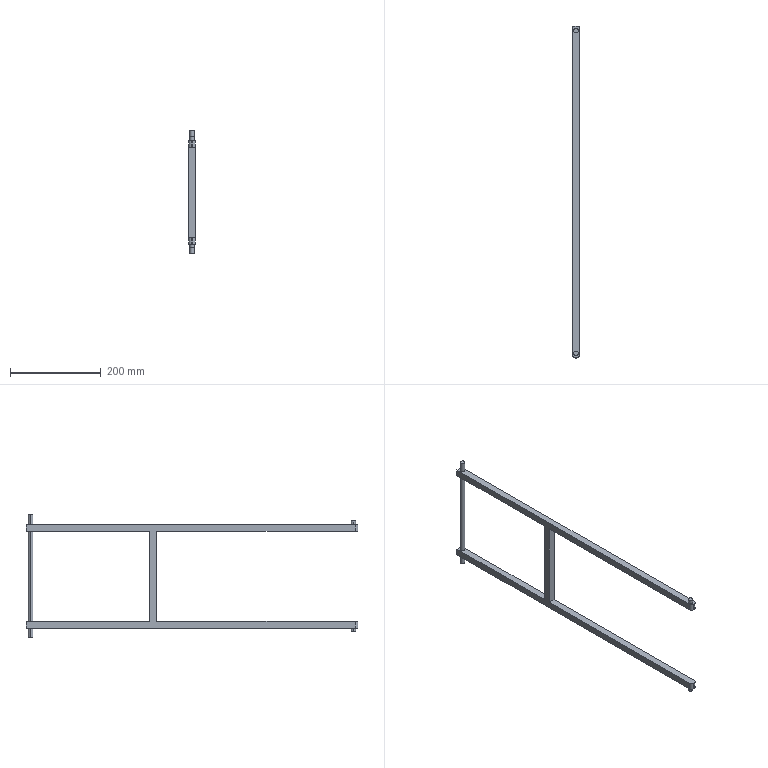Part | SolidWorks | features ICE 5, Extrusion 1, Fillet 1 | 1 solid | 32 faces | box 15 x 730 x 270 mm | volume 392693 mm3 | plane 18 | cylinder 14 | commonest cylinder face diameters 10 x10 12 x4
STEP:
#1=CARTESIAN_POINT('',(-5.,720.,-27.5));
#2=VERTEX_POINT('',#1);
#3=CARTESIAN_POINT('',(5.,720.,-27.5));
#4=VERTEX_POINT('',#3);
#5=CARTESIAN_POINT('',(0.,720.,-27.5));
#6=DIRECTION('',(0.,0.,-1.));
#7=DIRECTION('',(-1.,0.,0.));
#8=AXIS2_PLACEMENT_3D('',#5,#6,#7);
#9=CIRCLE('',#8,5.);
#10=EDGE_CURVE('',#2,#4,#9,.T.);
#11=ORIENTED_EDGE('',*,*,#10,.F.);
#12=CARTESIAN_POINT('',(-5.,720.,-7.5));
#13=VERTEX_POINT('',#12);
#14=CARTESIAN_POINT('',(-5.,720.,-27.5));
#15=DIRECTION('',(0.,0.,1.));
#16=VECTOR('',#15,1000.);
#17=LINE('',#14,#16);
#18=EDGE_CURVE('',#2,#13,#17,.T.);
#19=ORIENTED_EDGE('',*,*,#18,.T.);
#20=CARTESIAN_POINT('',(5.,720.,-7.5));
#21=VERTEX_POINT('',#20);
#22=CARTESIAN_POINT('',(0.,720.,-7.5));
#23=DIRECTION('',(0.,0.,-1.));
#24=DIRECTION('',(1.,0.,0.));
#25=AXIS2_PLACEMENT_3D('',#22,#23,#24);
#26=CIRCLE('',#25,5.);
#27=EDGE_CURVE('',#13,#21,#26,.T.);
#28=ORIENTED_EDGE('',*,*,#27,.T.);
#29=CARTESIAN_POINT('',(5.,720.,-27.5));
#30=DIRECTION('',(0.,0.,1.));
#31=VECTOR('',#30,1000.);
#32=LINE('',#29,#31);
#33=EDGE_CURVE('',#4,#21,#32,.T.);
#34=ORIENTED_EDGE('',*,*,#33,.F.);
#35=EDGE_LOOP('',(#11,#19,#28,#34));
#36=FACE_OUTER_BOUND('',#35,.T.);
#37=CARTESIAN_POINT('',(0.,720.,-27.5));
#38=DIRECTION('',(0.,0.,1.));
#39=DIRECTION('',(1.,0.,0.));
#40=AXIS2_PLACEMENT_3D('',#37,#38,#39);
#41=CYLINDRICAL_SURFACE('',#40,5.);
#42=ADVANCED_FACE('',(#36),#41,.T.);
#43=CARTESIAN_POINT('',(5.,720.,7.5));
#44=VERTEX_POINT('',#43);
#45=CARTESIAN_POINT('',(-5.,720.,7.5));
#46=VERTEX_POINT('',#45);
#47=CARTESIAN_POINT('',(0.,720.,7.5));
#48=DIRECTION('',(0.,0.,1.));
#49=DIRECTION('',(-1.,0.,0.));
#50=AXIS2_PLACEMENT_3D('',#47,#48,#49);
#51=CIRCLE('',#50,5.);
#52=EDGE_CURVE('',#44,#46,#51,.T.);
#53=ORIENTED_EDGE('',*,*,#52,.T.);
#54=CARTESIAN_POINT('',(-5.,720.,205.5));
#55=VERTEX_POINT('',#54);
#56=CARTESIAN_POINT('',(-5.,720.,-27.5));
#57=DIRECTION('',(0.,0.,1.));
#58=VECTOR('',#57,1000.);
#59=LINE('',#56,#58);
#60=EDGE_CURVE('',#46,#55,#59,.T.);
#61=ORIENTED_EDGE('',*,*,#60,.T.);
#62=CARTESIAN_POINT('',(5.,720.,205.5));
#63=VERTEX_POINT('',#62);
#64=CARTESIAN_POINT('',(0.,720.,205.5));
#65=DIRECTION('',(0.,0.,-1.));
#66=DIRECTION('',(1.,0.,0.));
#67=AXIS2_PLACEMENT_3D('',#64,#65,#66);
#68=CIRCLE('',#67,5.);
#69=EDGE_CURVE('',#55,#63,#68,.T.);
#70=ORIENTED_EDGE('',*,*,#69,.T.);
#71=CARTESIAN_POINT('',(5.,720.,-27.5));
#72=DIRECTION('',(0.,0.,1.));
#73=VECTOR('',#72,1000.);
#74=LINE('',#71,#73);
#75=EDGE_CURVE('',#44,#63,#74,.T.);
#76=ORIENTED_EDGE('',*,*,#75,.F.);
#77=EDGE_LOOP('',(#53,#61,#70,#76));
#78=FACE_OUTER_BOUND('',#77,.T.);
#79=CARTESIAN_POINT('',(0.,720.,-27.5));
#80=DIRECTION('',(0.,0.,1.));
#81=DIRECTION('',(1.,0.,0.));
#82=AXIS2_PLACEMENT_3D('',#79,#80,#81);
#83=CYLINDRICAL_SURFACE('',#82,5.);
#84=ADVANCED_FACE('',(#78),#83,.T.);
#85=CARTESIAN_POINT('',(-5.,720.,220.5));
#86=VERTEX_POINT('',#85);
#87=CARTESIAN_POINT('',(5.,720.,220.5));
#88=VERTEX_POINT('',#87);
#89=CARTESIAN_POINT('',(0.,720.,220.5));
#90=DIRECTION('',(0.,0.,-1.));
#91=DIRECTION('',(1.,0.,0.));
#92=AXIS2_PLACEMENT_3D('',#89,#90,#91);
#93=CIRCLE('',#92,5.);
#94=EDGE_CURVE('',#86,#88,#93,.T.);
#95=ORIENTED_EDGE('',*,*,#94,.F.);
#96=CARTESIAN_POINT('',(-5.,720.,242.5));
#97=VERTEX_POINT('',#96);
#98=CARTESIAN_POINT('',(-5.,720.,-27.5));
#99=DIRECTION('',(0.,0.,1.));
#100=VECTOR('',#99,1000.);
#101=LINE('',#98,#100);
#102=EDGE_CURVE('',#86,#97,#101,.T.);
#103=ORIENTED_EDGE('',*,*,#102,.T.);
#104=CARTESIAN_POINT('',(5.,720.,242.5));
#105=VERTEX_POINT('',#104);
#106=CARTESIAN_POINT('',(0.,720.,242.5));
#107=DIRECTION('',(0.,0.,-1.));
#108=DIRECTION('',(-1.,0.,0.));
#109=AXIS2_PLACEMENT_3D('',#106,#107,#108);
#110=CIRCLE('',#109,5.);
#111=EDGE_CURVE('',#97,#105,#110,.T.);
#112=ORIENTED_EDGE('',*,*,#111,.T.);
#113=CARTESIAN_POINT('',(5.,720.,-27.5));
#114=DIRECTION('',(0.,0.,1.));
#115=VECTOR('',#114,1000.);
#116=LINE('',#113,#115);
#117=EDGE_CURVE('',#88,#105,#116,.T.);
#118=ORIENTED_EDGE('',*,*,#117,.F.);
#119=EDGE_LOOP('',(#95,#103,#112,#118));
#120=FACE_OUTER_BOUND('',#119,.T.);
#121=CARTESIAN_POINT('',(0.,720.,-27.5));
#122=DIRECTION('',(0.,0.,1.));
#123=DIRECTION('',(1.,0.,0.));
#124=AXIS2_PLACEMENT_3D('',#121,#122,#123);
#125=CYLINDRICAL_SURFACE('',#124,5.);
#126=ADVANCED_FACE('',(#120),#125,.T.);
#127=CARTESIAN_POINT('',(5.,10.,228.5));
#128=VERTEX_POINT('',#127);
#129=CARTESIAN_POINT('',(-5.,10.,228.5));
#130=VERTEX_POINT('',#129);
#131=CARTESIAN_POINT('',(0.,10.,228.5));
#132=DIRECTION('',(0.,0.,1.));
#133=DIRECTION('',(1.,0.,0.));
#134=AXIS2_PLACEMENT_3D('',#131,#132,#133);
#135=CIRCLE('',#134,5.);
#136=EDGE_CURVE('',#128,#130,#135,.T.);
#137=ORIENTED_EDGE('',*,*,#136,.F.);
#138=CARTESIAN_POINT('',(5.,10.,220.5));
#139=VERTEX_POINT('',#138);
#140=CARTESIAN_POINT('',(5.,10.,228.5));
#141=DIRECTION('',(0.,0.,-1.));
#142=VECTOR('',#141,1000.);
#143=LINE('',#140,#142);
#144=EDGE_CURVE('',#128,#139,#143,.T.);
#145=ORIENTED_EDGE('',*,*,#144,.T.);
#146=CARTESIAN_POINT('',(-5.,10.,220.5));
#147=VERTEX_POINT('',#146);
#148=CARTESIAN_POINT('',(0.,10.,220.5));
#149=DIRECTION('',(0.,0.,1.));
#150=DIRECTION('',(1.,0.,0.));
#151=AXIS2_PLACEMENT_3D('',#148,#149,#150);
#152=CIRCLE('',#151,5.);
#153=EDGE_CURVE('',#139,#147,#152,.T.);
#154=ORIENTED_EDGE('',*,*,#153,.T.);
#155=CARTESIAN_POINT('',(-5.,10.,228.5));
#156=DIRECTION('',(0.,0.,-1.));
#157=VECTOR('',#156,1000.);
#158=LINE('',#155,#157);
#159=EDGE_CURVE('',#130,#147,#158,.T.);
#160=ORIENTED_EDGE('',*,*,#159,.F.);
#161=EDGE_LOOP('',(#137,#145,#154,#160));
#162=FACE_OUTER_BOUND('',#161,.T.);
#163=CARTESIAN_POINT('',(0.,10.,228.5));
#164=DIRECTION('',(0.,0.,-1.));
#165=DIRECTION('',(-1.,0.,0.));
#166=AXIS2_PLACEMENT_3D('',#163,#164,#165);
#167=CYLINDRICAL_SURFACE('',#166,5.);
#168=ADVANCED_FACE('',(#162),#167,.T.);
#169=CARTESIAN_POINT('',(-5.,10.,-15.5));
#170=VERTEX_POINT('',#169);
#171=CARTESIAN_POINT('',(5.,10.,-15.5));
#172=VERTEX_POINT('',#171);
#173=CARTESIAN_POINT('',(0.,10.,-15.5));
#174=DIRECTION('',(0.,0.,-1.));
#175=DIRECTION('',(-1.,0.,0.));
#176=AXIS2_PLACEMENT_3D('',#173,#174,#175);
#177=CIRCLE('',#176,5.);
#178=EDGE_CURVE('',#170,#172,#177,.T.);
#179=ORIENTED_EDGE('',*,*,#178,.F.);
#180=CARTESIAN_POINT('',(-5.,10.,-7.5));
#181=VERTEX_POINT('',#180);
#182=CARTESIAN_POINT('',(-5.,10.,-15.5));
#183=DIRECTION('',(0.,0.,1.));
#184=VECTOR('',#183,1000.);
#185=LINE('',#182,#184);
#186=EDGE_CURVE('',#170,#181,#185,.T.);
#187=ORIENTED_EDGE('',*,*,#186,.T.);
#188=CARTESIAN_POINT('',(5.,10.,-7.5));
#189=VERTEX_POINT('',#188);
#190=CARTESIAN_POINT('',(0.,10.,-7.5));
#191=DIRECTION('',(0.,0.,-1.));
#192=DIRECTION('',(1.,0.,0.));
#193=AXIS2_PLACEMENT_3D('',#190,#191,#192);
#194=CIRCLE('',#193,5.);
#195=EDGE_CURVE('',#181,#189,#194,.T.);
#196=ORIENTED_EDGE('',*,*,#195,.T.);
#197=CARTESIAN_POINT('',(5.,10.,-15.5));
#198=DIRECTION('',(0.,0.,1.));
#199=VECTOR('',#198,1000.);
#200=LINE('',#197,#199);
#201=EDGE_CURVE('',#172,#189,#200,.T.);
#202=ORIENTED_EDGE('',*,*,#201,.F.);
#203=EDGE_LOOP('',(#179,#187,#196,#202));
#204=FACE_OUTER_BOUND('',#203,.T.);
#205=CARTESIAN_POINT('',(0.,10.,-15.5));
#206=DIRECTION('',(0.,0.,1.));
#207=DIRECTION('',(1.,0.,0.));
#208=AXIS2_PLACEMENT_3D('',#205,#206,#207);
#209=CYLINDRICAL_SURFACE('',#208,5.);
#210=ADVANCED_FACE('',(#204),#209,.T.);
#211=CARTESIAN_POINT('',(-7.5,442.5,7.5));
#212=VERTEX_POINT('',#211);
#213=CARTESIAN_POINT('',(-7.5,6.,7.5));
#214=VERTEX_POINT('',#213);
#215=CARTESIAN_POINT('',(-7.5,730.,7.5));
#216=DIRECTION('',(0.,-1.,0.));
#217=VECTOR('',#216,1000.);
#218=LINE('',#215,#217);
#219=EDGE_CURVE('',#212,#214,#218,.T.);
#220=ORIENTED_EDGE('',*,*,#219,.T.);
#221=CARTESIAN_POINT('',(-1.5,0.,7.5));
#222=VERTEX_POINT('',#221);
#223=CARTESIAN_POINT('',(-1.5,6.,7.5));
#224=DIRECTION('',(0.,0.,1.));
#225=DIRECTION('',(-1.,0.,0.));
#226=AXIS2_PLACEMENT_3D('',#223,#224,#225);
#227=CIRCLE('',#226,6.);
#228=EDGE_CURVE('',#214,#222,#227,.T.);
#229=ORIENTED_EDGE('',*,*,#228,.T.);
#230=CARTESIAN_POINT('',(1.5,0.,7.5));
#231=VERTEX_POINT('',#230);
#232=CARTESIAN_POINT('',(-7.5,0.,7.5));
#233=DIRECTION('',(1.,0.,0.));
#234=VECTOR('',#233,1000.);
#235=LINE('',#232,#234);
#236=EDGE_CURVE('',#222,#231,#235,.T.);
#237=ORIENTED_EDGE('',*,*,#236,.T.);
#238=CARTESIAN_POINT('',(7.5,6.,7.5));
#239=VERTEX_POINT('',#238);
#240=CARTESIAN_POINT('',(1.5,6.,7.5));
#241=DIRECTION('',(0.,0.,1.));
#242=DIRECTION('',(-1.,0.,0.));
#243=AXIS2_PLACEMENT_3D('',#240,#241,#242);
#244=CIRCLE('',#243,6.);
#245=EDGE_CURVE('',#231,#239,#244,.T.);
#246=ORIENTED_EDGE('',*,*,#245,.T.);
#247=CARTESIAN_POINT('',(7.5,442.5,7.5));
#248=VERTEX_POINT('',#247);
#249=CARTESIAN_POINT('',(7.5,730.,7.5));
#250=DIRECTION('',(0.,-1.,0.));
#251=VECTOR('',#250,1000.);
#252=LINE('',#249,#251);
#253=EDGE_CURVE('',#248,#239,#252,.T.);
#254=ORIENTED_EDGE('',*,*,#253,.F.);
#255=CARTESIAN_POINT('',(-7.5,442.5,7.5));
#256=DIRECTION('',(1.,0.,0.));
#257=VECTOR('',#256,1000.);
#258=LINE('',#255,#257);
#259=EDGE_CURVE('',#212,#248,#258,.T.);
#260=ORIENTED_EDGE('',*,*,#259,.F.);
#261=EDGE_LOOP('',(#220,#229,#237,#246,#254,#260));
#262=FACE_OUTER_BOUND('',#261,.T.);
#263=CARTESIAN_POINT('',(-7.5,730.,7.5));
#264=DIRECTION('',(0.,0.,-1.));
#265=DIRECTION('',(-1.,0.,0.));
#266=AXIS2_PLACEMENT_3D('',#263,#264,#265);
#267=PLANE('',#266);
#268=ADVANCED_FACE('',(#262),#267,.F.);
#269=ORIENTED_EDGE('',*,*,#52,.F.);
#270=CARTESIAN_POINT('',(0.,720.,7.5));
#271=DIRECTION('',(0.,0.,1.));
#272=DIRECTION('',(-1.,0.,0.));
#273=AXIS2_PLACEMENT_3D('',#270,#271,#272);
#274=CIRCLE('',#273,5.);
#275=EDGE_CURVE('',#46,#44,#274,.T.);
#276=ORIENTED_EDGE('',*,*,#275,.F.);
#277=EDGE_LOOP('',(#269,#276));
#278=FACE_BOUND('',#277,.T.);
#279=CARTESIAN_POINT('',(7.5,457.5,7.5));
#280=VERTEX_POINT('',#279);
#281=CARTESIAN_POINT('',(-7.5,457.5,7.5));
#282=VERTEX_POINT('',#281);
#283=CARTESIAN_POINT('',(-7.5,457.5,7.5));
#284=DIRECTION('',(-1.,0.,0.));
#285=VECTOR('',#284,1000.);
#286=LINE('',#283,#285);
#287=EDGE_CURVE('',#280,#282,#286,.T.);
#288=ORIENTED_EDGE('',*,*,#287,.F.);
#289=CARTESIAN_POINT('',(7.5,730.,7.5));
#290=VERTEX_POINT('',#289);
#291=CARTESIAN_POINT('',(7.5,730.,7.5));
#292=DIRECTION('',(0.,-1.,0.));
#293=VECTOR('',#292,1000.);
#294=LINE('',#291,#293);
#295=EDGE_CURVE('',#290,#280,#294,.T.);
#296=ORIENTED_EDGE('',*,*,#295,.F.);
#297=CARTESIAN_POINT('',(-7.5,730.,7.5));
#298=VERTEX_POINT('',#297);
#299=CARTESIAN_POINT('',(-7.5,730.,7.5));
#300=DIRECTION('',(1.,0.,0.));
#301=VECTOR('',#300,1000.);
#302=LINE('',#299,#301);
#303=EDGE_CURVE('',#298,#290,#302,.T.);
#304=ORIENTED_EDGE('',*,*,#303,.F.);
#305=CARTESIAN_POINT('',(-7.5,730.,7.5));
#306=DIRECTION('',(0.,-1.,0.));
#307=VECTOR('',#306,1000.);
#308=LINE('',#305,#307);
#309=EDGE_CURVE('',#298,#282,#308,.T.);
#310=ORIENTED_EDGE('',*,*,#309,.T.);
#311=EDGE_LOOP('',(#288,#296,#304,#310));
#312=FACE_OUTER_BOUND('',#311,.T.);
#313=CARTESIAN_POINT('',(-7.5,730.,7.5));
#314=DIRECTION('',(0.,0.,-1.));
#315=DIRECTION('',(-1.,0.,0.));
#316=AXIS2_PLACEMENT_3D('',#313,#314,#315);
#317=PLANE('',#316);
#318=ADVANCED_FACE('',(#278,#312),#317,.F.);
#319=ORIENTED_EDGE('',*,*,#253,.T.);
#320=CARTESIAN_POINT('',(7.5,6.,-7.5));
#321=VERTEX_POINT('',#320);
#322=CARTESIAN_POINT('',(7.5,6.,-7.5));
#323=DIRECTION('',(0.,0.,-1.));
#324=VECTOR('',#323,1000.);
#325=LINE('',#322,#324);
#326=EDGE_CURVE('',#239,#321,#325,.T.);
#327=ORIENTED_EDGE('',*,*,#326,.T.);
#328=CARTESIAN_POINT('',(7.5,730.,-7.5));
#329=VERTEX_POINT('',#328);
#330=CARTESIAN_POINT('',(7.5,730.,-7.5));
#331=DIRECTION('',(0.,-1.,0.));
#332=VECTOR('',#331,1000.);
#333=LINE('',#330,#332);
#334=EDGE_CURVE('',#329,#321,#333,.T.);
#335=ORIENTED_EDGE('',*,*,#334,.F.);
#336=CARTESIAN_POINT('',(7.5,730.,-7.5));
#337=DIRECTION('',(0.,0.,-1.));
#338=VECTOR('',#337,1000.);
#339=LINE('',#336,#338);
#340=EDGE_CURVE('',#290,#329,#339,.T.);
#341=ORIENTED_EDGE('',*,*,#340,.F.);
#342=ORIENTED_EDGE('',*,*,#295,.T.);
#343=CARTESIAN_POINT('',(7.5,457.5,205.5));
#344=VERTEX_POINT('',#343);
#345=CARTESIAN_POINT('',(7.5,457.5,205.5));
#346=DIRECTION('',(0.,0.,-1.));
#347=VECTOR('',#346,1000.);
#348=LINE('',#345,#347);
#349=EDGE_CURVE('',#344,#280,#348,.T.);
#350=ORIENTED_EDGE('',*,*,#349,.F.);
#351=CARTESIAN_POINT('',(7.5,730.,205.5));
#352=VERTEX_POINT('',#351);
#353=CARTESIAN_POINT('',(7.5,730.,205.5));
#354=DIRECTION('',(0.,1.,0.));
#355=VECTOR('',#354,1000.);
#356=LINE('',#353,#355);
#357=EDGE_CURVE('',#344,#352,#356,.T.);
#358=ORIENTED_EDGE('',*,*,#357,.T.);
#359=CARTESIAN_POINT('',(7.5,730.,220.5));
#360=VERTEX_POINT('',#359);
#361=CARTESIAN_POINT('',(7.5,730.,220.5));
#362=DIRECTION('',(0.,0.,-1.));
#363=VECTOR('',#362,1000.);
#364=LINE('',#361,#363);
#365=EDGE_CURVE('',#360,#352,#364,.T.);
#366=ORIENTED_EDGE('',*,*,#365,.F.);
#367=CARTESIAN_POINT('',(7.5,6.,220.5));
#368=VERTEX_POINT('',#367);
#369=CARTESIAN_POINT('',(7.5,730.,220.5));
#370=DIRECTION('',(0.,1.,0.));
#371=VECTOR('',#370,1000.);
#372=LINE('',#369,#371);
#373=EDGE_CURVE('',#368,#360,#372,.T.);
#374=ORIENTED_EDGE('',*,*,#373,.F.);
#375=CARTESIAN_POINT('',(7.5,6.,205.5));
#376=VERTEX_POINT('',#375);
#377=CARTESIAN_POINT('',(7.5,6.,-7.5));
#378=DIRECTION('',(0.,0.,-1.));
#379=VECTOR('',#378,1000.);
#380=LINE('',#377,#379);
#381=EDGE_CURVE('',#368,#376,#380,.T.);
#382=ORIENTED_EDGE('',*,*,#381,.T.);
#383=CARTESIAN_POINT('',(7.5,442.5,205.5));
#384=VERTEX_POINT('',#383);
#385=CARTESIAN_POINT('',(7.5,730.,205.5));
#386=DIRECTION('',(0.,1.,0.));
#387=VECTOR('',#386,1000.);
#388=LINE('',#385,#387);
#389=EDGE_CURVE('',#376,#384,#388,.T.);
#390=ORIENTED_EDGE('',*,*,#389,.T.);
#391=CARTESIAN_POINT('',(7.5,442.5,205.5));
#392=DIRECTION('',(0.,0.,-1.));
#393=VECTOR('',#392,1000.);
#394=LINE('',#391,#393);
#395=EDGE_CURVE('',#384,#248,#394,.T.);
#396=ORIENTED_EDGE('',*,*,#395,.T.);
#397=EDGE_LOOP('',(#319,#327,#335,#341,#342,#350,#358,#366,#374,#382,#390,#396));
#398=FACE_OUTER_BOUND('',#397,.T.);
#399=CARTESIAN_POINT('',(7.5,730.,-7.5));
#400=DIRECTION('',(-1.,0.,0.));
#401=DIRECTION('',(0.,0.,1.));
#402=AXIS2_PLACEMENT_3D('',#399,#400,#401);
#403=PLANE('',#402);
#404=ADVANCED_FACE('',(#398),#403,.F.);
#405=CARTESIAN_POINT('',(0.,720.,-7.5));
#406=DIRECTION('',(0.,0.,-1.));
#407=DIRECTION('',(1.,0.,0.));
#408=AXIS2_PLACEMENT_3D('',#405,#406,#407);
#409=CIRCLE('',#408,5.);
#410=EDGE_CURVE('',#21,#13,#409,.T.);
#411=ORIENTED_EDGE('',*,*,#410,.F.);
#412=ORIENTED_EDGE('',*,*,#27,.F.);
#413=EDGE_LOOP('',(#411,#412));
#414=FACE_BOUND('',#413,.T.);
#415=CARTESIAN_POINT('',(0.,10.,-7.5));
#416=DIRECTION('',(0.,0.,-1.));
#417=DIRECTION('',(1.,0.,0.));
#418=AXIS2_PLACEMENT_3D('',#415,#416,#417);
#419=CIRCLE('',#418,5.);
#420=EDGE_CURVE('',#189,#181,#419,.T.);
#421=ORIENTED_EDGE('',*,*,#420,.F.);
#422=ORIENTED_EDGE('',*,*,#195,.F.);
#423=EDGE_LOOP('',(#421,#422));
#424=FACE_BOUND('',#423,.T.);
#425=CARTESIAN_POINT('',(1.5,0.,-7.5));
#426=VERTEX_POINT('',#425);
#427=CARTESIAN_POINT('',(-1.5,0.,-7.5));
#428=VERTEX_POINT('',#427);
#429=CARTESIAN_POINT('',(-7.5,0.,-7.5));
#430=DIRECTION('',(-1.,0.,0.));
#431=VECTOR('',#430,1000.);
#432=LINE('',#429,#431);
#433=EDGE_CURVE('',#426,#428,#432,.T.);
#434=ORIENTED_EDGE('',*,*,#433,.T.);
#435=CARTESIAN_POINT('',(-7.5,6.,-7.5));
#436=VERTEX_POINT('',#435);
#437=CARTESIAN_POINT('',(-1.5,6.,-7.5));
#438=DIRECTION('',(0.,0.,-1.));
#439=DIRECTION('',(1.,0.,0.));
#440=AXIS2_PLACEMENT_3D('',#437,#438,#439);
#441=CIRCLE('',#440,6.);
#442=EDGE_CURVE('',#428,#436,#441,.T.);
#443=ORIENTED_EDGE('',*,*,#442,.T.);
#444=CARTESIAN_POINT('',(-7.5,730.,-7.5));
#445=VERTEX_POINT('',#444);
#446=CARTESIAN_POINT('',(-7.5,730.,-7.5));
#447=DIRECTION('',(0.,-1.,0.));
#448=VECTOR('',#447,1000.);
#449=LINE('',#446,#448);
#450=EDGE_CURVE('',#445,#436,#449,.T.);
#451=ORIENTED_EDGE('',*,*,#450,.F.);
#452=CARTESIAN_POINT('',(-7.5,730.,-7.5));
#453=DIRECTION('',(-1.,0.,0.));
#454=VECTOR('',#453,1000.);
#455=LINE('',#452,#454);
#456=EDGE_CURVE('',#329,#445,#455,.T.);
#457=ORIENTED_EDGE('',*,*,#456,.F.);
#458=ORIENTED_EDGE('',*,*,#334,.T.);
#459=CARTESIAN_POINT('',(1.5,6.,-7.5));
#460=DIRECTION('',(0.,0.,-1.));
#461=DIRECTION('',(1.,0.,0.));
#462=AXIS2_PLACEMENT_3D('',#459,#460,#461);
#463=CIRCLE('',#462,6.);
#464=EDGE_CURVE('',#321,#426,#463,.T.);
#465=ORIENTED_EDGE('',*,*,#464,.T.);
#466=EDGE_LOOP('',(#434,#443,#451,#457,#458,#465));
#467=FACE_OUTER_BOUND('',#466,.T.);
#468=CARTESIAN_POINT('',(-7.5,730.,-7.5));
#469=DIRECTION('',(0.,0.,1.));
#470=DIRECTION('',(1.,0.,0.));
#471=AXIS2_PLACEMENT_3D('',#468,#469,#470);
#472=PLANE('',#471);
#473=ADVANCED_FACE('',(#414,#424,#467),#472,.F.);
#474=ORIENTED_EDGE('',*,*,#450,.T.);
#475=CARTESIAN_POINT('',(-7.5,6.,-7.5));
#476=DIRECTION('',(0.,0.,1.));
#477=VECTOR('',#476,1000.);
#478=LINE('',#475,#477);
#479=EDGE_CURVE('',#436,#214,#478,.T.);
#480=ORIENTED_EDGE('',*,*,#479,.T.);
#481=ORIENTED_EDGE('',*,*,#219,.F.);
#482=CARTESIAN_POINT('',(-7.5,442.5,205.5));
#483=VERTEX_POINT('',#482);
#484=CARTESIAN_POINT('',(-7.5,442.5,205.5));
#485=DIRECTION('',(0.,0.,-1.));
#486=VECTOR('',#485,1000.);
#487=LINE('',#484,#486);
#488=EDGE_CURVE('',#483,#212,#487,.T.);
#489=ORIENTED_EDGE('',*,*,#488,.F.);
#490=CARTESIAN_POINT('',(-7.5,6.,205.5));
#491=VERTEX_POINT('',#490);
#492=CARTESIAN_POINT('',(-7.5,730.,205.5));
#493=DIRECTION('',(0.,-1.,0.));
#494=VECTOR('',#493,1000.);
#495=LINE('',#492,#494);
#496=EDGE_CURVE('',#483,#491,#495,.T.);
#497=ORIENTED_EDGE('',*,*,#496,.T.);
#498=CARTESIAN_POINT('',(-7.5,6.,220.5));
#499=VERTEX_POINT('',#498);
#500=CARTESIAN_POINT('',(-7.5,6.,-7.5));
#501=DIRECTION('',(0.,0.,1.));
#502=VECTOR('',#501,1000.);
#503=LINE('',#500,#502);
#504=EDGE_CURVE('',#491,#499,#503,.T.);
#505=ORIENTED_EDGE('',*,*,#504,.T.);
#506=CARTESIAN_POINT('',(-7.5,730.,220.5));
#507=VERTEX_POINT('',#506);
#508=CARTESIAN_POINT('',(-7.5,730.,220.5));
#509=DIRECTION('',(0.,-1.,0.));
#510=VECTOR('',#509,1000.);
#511=LINE('',#508,#510);
#512=EDGE_CURVE('',#507,#499,#511,.T.);
#513=ORIENTED_EDGE('',*,*,#512,.F.);
#514=CARTESIAN_POINT('',(-7.5,730.,205.5));
#515=VERTEX_POINT('',#514);
#516=CARTESIAN_POINT('',(-7.5,730.,220.5));
#517=DIRECTION('',(0.,0.,-1.));
#518=VECTOR('',#517,1000.);
#519=LINE('',#516,#518);
#520=EDGE_CURVE('',#507,#515,#519,.T.);
#521=ORIENTED_EDGE('',*,*,#520,.T.);
#522=CARTESIAN_POINT('',(-7.5,457.5,205.5));
#523=VERTEX_POINT('',#522);
#524=CARTESIAN_POINT('',(-7.5,730.,205.5));
#525=DIRECTION('',(0.,-1.,0.));
#526=VECTOR('',#525,1000.);
#527=LINE('',#524,#526);
#528=EDGE_CURVE('',#515,#523,#527,.T.);
#529=ORIENTED_EDGE('',*,*,#528,.T.);
#530=CARTESIAN_POINT('',(-7.5,457.5,205.5));
#531=DIRECTION('',(0.,0.,-1.));
#532=VECTOR('',#531,1000.);
#533=LINE('',#530,#532);
#534=EDGE_CURVE('',#523,#282,#533,.T.);
#535=ORIENTED_EDGE('',*,*,#534,.T.);
#536=ORIENTED_EDGE('',*,*,#309,.F.);
#537=CARTESIAN_POINT('',(-7.5,730.,-7.5));
#538=DIRECTION('',(0.,0.,1.));
#539=VECTOR('',#538,1000.);
#540=LINE('',#537,#539);
#541=EDGE_CURVE('',#445,#298,#540,.T.);
#542=ORIENTED_EDGE('',*,*,#541,.F.);
#543=EDGE_LOOP('',(#474,#480,#481,#489,#497,#505,#513,#521,#529,#535,#536,#542));
#544=FACE_OUTER_BOUND('',#543,.T.);
#545=CARTESIAN_POINT('',(-7.5,730.,-7.5));
#546=DIRECTION('',(1.,0.,0.));
#547=DIRECTION('',(0.,0.,-1.));
#548=AXIS2_PLACEMENT_3D('',#545,#546,#547);
#549=PLANE('',#548);
#550=ADVANCED_FACE('',(#544),#549,.F.);
#551=ORIENTED_EDGE('',*,*,#340,.T.);
#552=ORIENTED_EDGE('',*,*,#456,.T.);
#553=ORIENTED_EDGE('',*,*,#541,.T.);
#554=ORIENTED_EDGE('',*,*,#303,.T.);
#555=EDGE_LOOP('',(#551,#552,#553,#554));
#556=FACE_OUTER_BOUND('',#555,.T.);
#557=CARTESIAN_POINT('',(0.,730.,0.));
#558=DIRECTION('',(0.,1.,0.));
#559=DIRECTION('',(0.,0.,1.));
#560=AXIS2_PLACEMENT_3D('',#557,#558,#559);
#561=PLANE('',#560);
#562=ADVANCED_FACE('',(#556),#561,.T.);
#563=ORIENTED_EDGE('',*,*,#236,.F.);
#564=CARTESIAN_POINT('',(-1.5,0.,0.));
#565=DIRECTION('',(0.,0.,-1.));
#566=VECTOR('',#565,1000.);
#567=LINE('',#564,#566);
#568=EDGE_CURVE('',#222,#428,#567,.T.);
#569=ORIENTED_EDGE('',*,*,#568,.T.);
#570=ORIENTED_EDGE('',*,*,#433,.F.);
#571=CARTESIAN_POINT('',(1.5,0.,0.));
#572=DIRECTION('',(0.,0.,1.));
#573=VECTOR('',#572,1000.);
#574=LINE('',#571,#573);
#575=EDGE_CURVE('',#426,#231,#574,.T.);
#576=ORIENTED_EDGE('',*,*,#575,.T.);
#577=EDGE_LOOP('',(#563,#569,#570,#576));
#578=FACE_OUTER_BOUND('',#577,.T.);
#579=CARTESIAN_POINT('',(0.,0.,0.));
#580=DIRECTION('',(0.,1.,0.));
#581=DIRECTION('',(0.,0.,1.));
#582=AXIS2_PLACEMENT_3D('',#579,#580,#581);
#583=PLANE('',#582);
#584=ADVANCED_FACE('',(#578),#583,.F.);
#585=ORIENTED_EDGE('',*,*,#186,.F.);
#586=CARTESIAN_POINT('',(0.,10.,-15.5));
#587=DIRECTION('',(0.,0.,-1.));
#588=DIRECTION('',(-1.,0.,0.));
#589=AXIS2_PLACEMENT_3D('',#586,#587,#588);
#590=CIRCLE('',#589,5.);
#591=EDGE_CURVE('',#172,#170,#590,.T.);
#592=ORIENTED_EDGE('',*,*,#591,.F.);
#593=ORIENTED_EDGE('',*,*,#201,.T.);
#594=ORIENTED_EDGE('',*,*,#420,.T.);
#595=EDGE_LOOP('',(#585,#592,#593,#594));
#596=FACE_OUTER_BOUND('',#595,.T.);
#597=CARTESIAN_POINT('',(0.,10.,-15.5));
#598=DIRECTION('',(0.,0.,1.));
#599=DIRECTION('',(1.,0.,0.));
#600=AXIS2_PLACEMENT_3D('',#597,#598,#599);
#601=CYLINDRICAL_SURFACE('',#600,5.);
#602=ADVANCED_FACE('',(#596),#601,.T.);
#603=ORIENTED_EDGE('',*,*,#591,.T.);
#604=ORIENTED_EDGE('',*,*,#178,.T.);
#605=EDGE_LOOP('',(#603,#604));
#606=FACE_OUTER_BOUND('',#605,.T.);
#607=CARTESIAN_POINT('',(0.,10.,-15.5));
#608=DIRECTION('',(0.,0.,-1.));
#609=DIRECTION('',(-1.,0.,0.));
#610=AXIS2_PLACEMENT_3D('',#607,#608,#609);
#611=PLANE('',#610);
#612=ADVANCED_FACE('',(#606),#611,.T.);
#613=ORIENTED_EDGE('',*,*,#287,.T.);
#614=ORIENTED_EDGE('',*,*,#534,.F.);
#615=CARTESIAN_POINT('',(-7.5,457.5,205.5));
#616=DIRECTION('',(-1.,0.,0.));
#617=VECTOR('',#616,1000.);
#618=LINE('',#615,#617);
#619=EDGE_CURVE('',#344,#523,#618,.T.);
#620=ORIENTED_EDGE('',*,*,#619,.F.);
#621=ORIENTED_EDGE('',*,*,#349,.T.);
#622=EDGE_LOOP('',(#613,#614,#620,#621));
#623=FACE_OUTER_BOUND('',#622,.T.);
#624=CARTESIAN_POINT('',(-7.5,457.5,205.5));
#625=DIRECTION('',(0.,-1.,0.));
#626=DIRECTION('',(0.,0.,-1.));
#627=AXIS2_PLACEMENT_3D('',#624,#625,#626);
#628=PLANE('',#627);
#629=ADVANCED_FACE('',(#623),#628,.F.);
#630=ORIENTED_EDGE('',*,*,#259,.T.);
#631=ORIENTED_EDGE('',*,*,#395,.F.);
#632=CARTESIAN_POINT('',(-7.5,442.5,205.5));
#633=DIRECTION('',(1.,0.,0.));
#634=VECTOR('',#633,1000.);
#635=LINE('',#632,#634);
#636=EDGE_CURVE('',#483,#384,#635,.T.);
#637=ORIENTED_EDGE('',*,*,#636,.F.);
#638=ORIENTED_EDGE('',*,*,#488,.T.);
#639=EDGE_LOOP('',(#630,#631,#637,#638));
#640=FACE_OUTER_BOUND('',#639,.T.);
#641=CARTESIAN_POINT('',(-7.5,442.5,205.5));
#642=DIRECTION('',(0.,1.,0.));
#643=DIRECTION('',(0.,0.,1.));
#644=AXIS2_PLACEMENT_3D('',#641,#642,#643);
#645=PLANE('',#644);
#646=ADVANCED_FACE('',(#640),#645,.F.);
#647=CARTESIAN_POINT('',(0.,720.,205.5));
#648=DIRECTION('',(0.,0.,-1.));
#649=DIRECTION('',(1.,0.,0.));
#650=AXIS2_PLACEMENT_3D('',#647,#648,#649);
#651=CIRCLE('',#650,5.);
#652=EDGE_CURVE('',#63,#55,#651,.T.);
#653=ORIENTED_EDGE('',*,*,#652,.F.);
#654=ORIENTED_EDGE('',*,*,#69,.F.);
#655=EDGE_LOOP('',(#653,#654));
#656=FACE_BOUND('',#655,.T.);
#657=ORIENTED_EDGE('',*,*,#357,.F.);
#658=ORIENTED_EDGE('',*,*,#619,.T.);
#659=ORIENTED_EDGE('',*,*,#528,.F.);
#660=CARTESIAN_POINT('',(-7.5,730.,205.5));
#661=DIRECTION('',(-1.,0.,0.));
#662=VECTOR('',#661,1000.);
#663=LINE('',#660,#662);
#664=EDGE_CURVE('',#352,#515,#663,.T.);
#665=ORIENTED_EDGE('',*,*,#664,.F.);
#666=EDGE_LOOP('',(#657,#658,#659,#665));
#667=FACE_OUTER_BOUND('',#666,.T.);
#668=CARTESIAN_POINT('',(0.,0.,205.5));
#669=DIRECTION('',(0.,0.,1.));
#670=DIRECTION('',(1.,0.,0.));
#671=AXIS2_PLACEMENT_3D('',#668,#669,#670);
#672=PLANE('',#671);
#673=ADVANCED_FACE('',(#656,#667),#672,.F.);
#674=CARTESIAN_POINT('',(-1.5,0.,205.5));
#675=VERTEX_POINT('',#674);
#676=CARTESIAN_POINT('',(1.5,0.,205.5));
#677=VERTEX_POINT('',#676);
#678=CARTESIAN_POINT('',(-7.5,0.,205.5));
#679=DIRECTION('',(1.,0.,0.));
#680=VECTOR('',#679,1000.);
#681=LINE('',#678,#680);
#682=EDGE_CURVE('',#675,#677,#681,.T.);
#683=ORIENTED_EDGE('',*,*,#682,.F.);
#684=CARTESIAN_POINT('',(-1.5,6.,205.5));
#685=DIRECTION('',(0.,0.,-1.));
#686=DIRECTION('',(1.,0.,0.));
#687=AXIS2_PLACEMENT_3D('',#684,#685,#686);
#688=CIRCLE('',#687,6.);
#689=EDGE_CURVE('',#675,#491,#688,.T.);
#690=ORIENTED_EDGE('',*,*,#689,.T.);
#691=ORIENTED_EDGE('',*,*,#496,.F.);
#692=ORIENTED_EDGE('',*,*,#636,.T.);
#693=ORIENTED_EDGE('',*,*,#389,.F.);
#694=CARTESIAN_POINT('',(1.5,6.,205.5));
#695=DIRECTION('',(0.,0.,-1.));
#696=DIRECTION('',(1.,0.,0.));
#697=AXIS2_PLACEMENT_3D('',#694,#695,#696);
#698=CIRCLE('',#697,6.);
#699=EDGE_CURVE('',#376,#677,#698,.T.);
#700=ORIENTED_EDGE('',*,*,#699,.T.);
#701=EDGE_LOOP('',(#683,#690,#691,#692,#693,#700));
#702=FACE_OUTER_BOUND('',#701,.T.);
#703=CARTESIAN_POINT('',(0.,0.,205.5));
#704=DIRECTION('',(0.,0.,1.));
#705=DIRECTION('',(1.,0.,0.));
#706=AXIS2_PLACEMENT_3D('',#703,#704,#705);
#707=PLANE('',#706);
#708=ADVANCED_FACE('',(#702),#707,.F.);
#709=ORIENTED_EDGE('',*,*,#664,.T.);
#710=ORIENTED_EDGE('',*,*,#520,.F.);
#711=CARTESIAN_POINT('',(-7.5,730.,220.5));
#712=DIRECTION('',(-1.,0.,0.));
#713=VECTOR('',#712,1000.);
#714=LINE('',#711,#713);
#715=EDGE_CURVE('',#360,#507,#714,.T.);
#716=ORIENTED_EDGE('',*,*,#715,.F.);
#717=ORIENTED_EDGE('',*,*,#365,.T.);
#718=EDGE_LOOP('',(#709,#710,#716,#717));
#719=FACE_OUTER_BOUND('',#718,.T.);
#720=CARTESIAN_POINT('',(-7.5,730.,220.5));
#721=DIRECTION('',(0.,-1.,0.));
#722=DIRECTION('',(0.,0.,-1.));
#723=AXIS2_PLACEMENT_3D('',#720,#721,#722);
#724=PLANE('',#723);
#725=ADVANCED_FACE('',(#719),#724,.F.);
#726=CARTESIAN_POINT('',(-1.5,0.,220.5));
#727=VERTEX_POINT('',#726);
#728=CARTESIAN_POINT('',(1.5,0.,220.5));
#729=VERTEX_POINT('',#728);
#730=CARTESIAN_POINT('',(-7.5,0.,220.5));
#731=DIRECTION('',(1.,0.,0.));
#732=VECTOR('',#731,1000.);
#733=LINE('',#730,#732);
#734=EDGE_CURVE('',#727,#729,#733,.T.);
#735=ORIENTED_EDGE('',*,*,#734,.F.);
#736=CARTESIAN_POINT('',(-1.5,0.,220.5));
#737=DIRECTION('',(0.,0.,-1.));
#738=VECTOR('',#737,1000.);
#739=LINE('',#736,#738);
#740=EDGE_CURVE('',#727,#675,#739,.T.);
#741=ORIENTED_EDGE('',*,*,#740,.T.);
#742=ORIENTED_EDGE('',*,*,#682,.T.);
#743=CARTESIAN_POINT('',(1.5,0.,220.5));
#744=DIRECTION('',(0.,0.,1.));
#745=VECTOR('',#744,1000.);
#746=LINE('',#743,#745);
#747=EDGE_CURVE('',#677,#729,#746,.T.);
#748=ORIENTED_EDGE('',*,*,#747,.T.);
#749=EDGE_LOOP('',(#735,#741,#742,#748));
#750=FACE_OUTER_BOUND('',#749,.T.);
#751=CARTESIAN_POINT('',(-7.5,0.,220.5));
#752=DIRECTION('',(0.,1.,0.));
#753=DIRECTION('',(0.,0.,1.));
#754=AXIS2_PLACEMENT_3D('',#751,#752,#753);
#755=PLANE('',#754);
#756=ADVANCED_FACE('',(#750),#755,.F.);
#757=CARTESIAN_POINT('',(0.,720.,220.5));
#758=DIRECTION('',(0.,0.,-1.));
#759=DIRECTION('',(1.,0.,0.));
#760=AXIS2_PLACEMENT_3D('',#757,#758,#759);
#761=CIRCLE('',#760,5.);
#762=EDGE_CURVE('',#88,#86,#761,.T.);
#763=ORIENTED_EDGE('',*,*,#762,.T.);
#764=ORIENTED_EDGE('',*,*,#94,.T.);
#765=EDGE_LOOP('',(#763,#764));
#766=FACE_BOUND('',#765,.T.);
#767=CARTESIAN_POINT('',(0.,10.,220.5));
#768=DIRECTION('',(0.,0.,1.));
#769=DIRECTION('',(1.,0.,0.));
#770=AXIS2_PLACEMENT_3D('',#767,#768,#769);
#771=CIRCLE('',#770,5.);
#772=EDGE_CURVE('',#147,#139,#771,.T.);
#773=ORIENTED_EDGE('',*,*,#772,.F.);
#774=ORIENTED_EDGE('',*,*,#153,.F.);
#775=EDGE_LOOP('',(#773,#774));
#776=FACE_BOUND('',#775,.T.);
#777=ORIENTED_EDGE('',*,*,#512,.T.);
#778=CARTESIAN_POINT('',(-1.5,6.,220.5));
#779=DIRECTION('',(0.,0.,1.));
#780=DIRECTION('',(1.,0.,0.));
#781=AXIS2_PLACEMENT_3D('',#778,#779,#780);
#782=CIRCLE('',#781,6.);
#783=EDGE_CURVE('',#499,#727,#782,.T.);
#784=ORIENTED_EDGE('',*,*,#783,.T.);
#785=ORIENTED_EDGE('',*,*,#734,.T.);
#786=CARTESIAN_POINT('',(1.5,6.,220.5));
#787=DIRECTION('',(0.,0.,1.));
#788=DIRECTION('',(1.,0.,0.));
#789=AXIS2_PLACEMENT_3D('',#786,#787,#788);
#790=CIRCLE('',#789,6.);
#791=EDGE_CURVE('',#729,#368,#790,.T.);
#792=ORIENTED_EDGE('',*,*,#791,.T.);
#793=ORIENTED_EDGE('',*,*,#373,.T.);
#794=ORIENTED_EDGE('',*,*,#715,.T.);
#795=EDGE_LOOP('',(#777,#784,#785,#792,#793,#794));
#796=FACE_OUTER_BOUND('',#795,.T.);
#797=CARTESIAN_POINT('',(0.,0.,220.5));
#798=DIRECTION('',(0.,0.,1.));
#799=DIRECTION('',(1.,0.,0.));
#800=AXIS2_PLACEMENT_3D('',#797,#798,#799);
#801=PLANE('',#800);
#802=ADVANCED_FACE('',(#766,#776,#796),#801,.T.);
#803=ORIENTED_EDGE('',*,*,#144,.F.);
#804=CARTESIAN_POINT('',(0.,10.,228.5));
#805=DIRECTION('',(0.,0.,1.));
#806=DIRECTION('',(1.,0.,0.));
#807=AXIS2_PLACEMENT_3D('',#804,#805,#806);
#808=CIRCLE('',#807,5.);
#809=EDGE_CURVE('',#130,#128,#808,.T.);
#810=ORIENTED_EDGE('',*,*,#809,.F.);
#811=ORIENTED_EDGE('',*,*,#159,.T.);
#812=ORIENTED_EDGE('',*,*,#772,.T.);
#813=EDGE_LOOP('',(#803,#810,#811,#812));
#814=FACE_OUTER_BOUND('',#813,.T.);
#815=CARTESIAN_POINT('',(0.,10.,228.5));
#816=DIRECTION('',(0.,0.,-1.));
#817=DIRECTION('',(-1.,0.,0.));
#818=AXIS2_PLACEMENT_3D('',#815,#816,#817);
#819=CYLINDRICAL_SURFACE('',#818,5.);
#820=ADVANCED_FACE('',(#814),#819,.T.);
#821=ORIENTED_EDGE('',*,*,#809,.T.);
#822=ORIENTED_EDGE('',*,*,#136,.T.);
#823=EDGE_LOOP('',(#821,#822));
#824=FACE_OUTER_BOUND('',#823,.T.);
#825=CARTESIAN_POINT('',(0.,10.,228.5));
#826=DIRECTION('',(0.,0.,1.));
#827=DIRECTION('',(1.,0.,0.));
#828=AXIS2_PLACEMENT_3D('',#825,#826,#827);
#829=PLANE('',#828);
#830=ADVANCED_FACE('',(#824),#829,.T.);
#831=ORIENTED_EDGE('',*,*,#442,.F.);
#832=ORIENTED_EDGE('',*,*,#568,.F.);
#833=ORIENTED_EDGE('',*,*,#228,.F.);
#834=ORIENTED_EDGE('',*,*,#479,.F.);
#835=EDGE_LOOP('',(#831,#832,#833,#834));
#836=FACE_OUTER_BOUND('',#835,.T.);
#837=CARTESIAN_POINT('',(-1.5,6.,-7.5));
#838=DIRECTION('',(0.,0.,1.));
#839=DIRECTION('',(1.,0.,0.));
#840=AXIS2_PLACEMENT_3D('',#837,#838,#839);
#841=CYLINDRICAL_SURFACE('',#840,6.);
#842=ADVANCED_FACE('',(#836),#841,.T.);
#843=ORIENTED_EDGE('',*,*,#245,.F.);
#844=ORIENTED_EDGE('',*,*,#575,.F.);
#845=ORIENTED_EDGE('',*,*,#464,.F.);
#846=ORIENTED_EDGE('',*,*,#326,.F.);
#847=EDGE_LOOP('',(#843,#844,#845,#846));
#848=FACE_OUTER_BOUND('',#847,.T.);
#849=CARTESIAN_POINT('',(1.5,6.,-7.5));
#850=DIRECTION('',(0.,0.,-1.));
#851=DIRECTION('',(-1.,0.,0.));
#852=AXIS2_PLACEMENT_3D('',#849,#850,#851);
#853=CYLINDRICAL_SURFACE('',#852,6.);
#854=ADVANCED_FACE('',(#848),#853,.T.);
#855=ORIENTED_EDGE('',*,*,#783,.F.);
#856=ORIENTED_EDGE('',*,*,#504,.F.);
#857=ORIENTED_EDGE('',*,*,#689,.F.);
#858=ORIENTED_EDGE('',*,*,#740,.F.);
#859=EDGE_LOOP('',(#855,#856,#857,#858));
#860=FACE_OUTER_BOUND('',#859,.T.);
#861=CARTESIAN_POINT('',(-1.5,6.,220.5));
#862=DIRECTION('',(0.,0.,-1.));
#863=DIRECTION('',(-1.,0.,0.));
#864=AXIS2_PLACEMENT_3D('',#861,#862,#863);
#865=CYLINDRICAL_SURFACE('',#864,6.);
#866=ADVANCED_FACE('',(#860),#865,.T.);
#867=ORIENTED_EDGE('',*,*,#791,.F.);
#868=ORIENTED_EDGE('',*,*,#747,.F.);
#869=ORIENTED_EDGE('',*,*,#699,.F.);
#870=ORIENTED_EDGE('',*,*,#381,.F.);
#871=EDGE_LOOP('',(#867,#868,#869,#870));
#872=FACE_OUTER_BOUND('',#871,.T.);
#873=CARTESIAN_POINT('',(1.5,6.,-7.5));
#874=DIRECTION('',(0.,0.,-1.));
#875=DIRECTION('',(-1.,0.,0.));
#876=AXIS2_PLACEMENT_3D('',#873,#874,#875);
#877=CYLINDRICAL_SURFACE('',#876,6.);
#878=ADVANCED_FACE('',(#872),#877,.T.);
#879=CARTESIAN_POINT('',(0.,720.,242.5));
#880=DIRECTION('',(0.,0.,-1.));
#881=DIRECTION('',(-1.,0.,0.));
#882=AXIS2_PLACEMENT_3D('',#879,#880,#881);
#883=CIRCLE('',#882,5.);
#884=EDGE_CURVE('',#105,#97,#883,.T.);
#885=ORIENTED_EDGE('',*,*,#884,.F.);
#886=ORIENTED_EDGE('',*,*,#111,.F.);
#887=EDGE_LOOP('',(#885,#886));
#888=FACE_OUTER_BOUND('',#887,.T.);
#889=CARTESIAN_POINT('',(0.,720.,242.5));
#890=DIRECTION('',(0.,0.,-1.));
#891=DIRECTION('',(-1.,0.,0.));
#892=AXIS2_PLACEMENT_3D('',#889,#890,#891);
#893=PLANE('',#892);
#894=ADVANCED_FACE('',(#888),#893,.F.);
#895=ORIENTED_EDGE('',*,*,#102,.F.);
#896=ORIENTED_EDGE('',*,*,#762,.F.);
#897=ORIENTED_EDGE('',*,*,#117,.T.);
#898=ORIENTED_EDGE('',*,*,#884,.T.);
#899=EDGE_LOOP('',(#895,#896,#897,#898));
#900=FACE_OUTER_BOUND('',#899,.T.);
#901=CARTESIAN_POINT('',(0.,720.,-27.5));
#902=DIRECTION('',(0.,0.,1.));
#903=DIRECTION('',(1.,0.,0.));
#904=AXIS2_PLACEMENT_3D('',#901,#902,#903);
#905=CYLINDRICAL_SURFACE('',#904,5.);
#906=ADVANCED_FACE('',(#900),#905,.T.);
#907=ORIENTED_EDGE('',*,*,#60,.F.);
#908=ORIENTED_EDGE('',*,*,#275,.T.);
#909=ORIENTED_EDGE('',*,*,#75,.T.);
#910=ORIENTED_EDGE('',*,*,#652,.T.);
#911=EDGE_LOOP('',(#907,#908,#909,#910));
#912=FACE_OUTER_BOUND('',#911,.T.);
#913=CARTESIAN_POINT('',(0.,720.,-27.5));
#914=DIRECTION('',(0.,0.,1.));
#915=DIRECTION('',(1.,0.,0.));
#916=AXIS2_PLACEMENT_3D('',#913,#914,#915);
#917=CYLINDRICAL_SURFACE('',#916,5.);
#918=ADVANCED_FACE('',(#912),#917,.T.);
#919=ORIENTED_EDGE('',*,*,#18,.F.);
#920=CARTESIAN_POINT('',(0.,720.,-27.5));
#921=DIRECTION('',(0.,0.,-1.));
#922=DIRECTION('',(-1.,0.,0.));
#923=AXIS2_PLACEMENT_3D('',#920,#921,#922);
#924=CIRCLE('',#923,5.);
#925=EDGE_CURVE('',#4,#2,#924,.T.);
#926=ORIENTED_EDGE('',*,*,#925,.F.);
#927=ORIENTED_EDGE('',*,*,#33,.T.);
#928=ORIENTED_EDGE('',*,*,#410,.T.);
#929=EDGE_LOOP('',(#919,#926,#927,#928));
#930=FACE_OUTER_BOUND('',#929,.T.);
#931=CARTESIAN_POINT('',(0.,720.,-27.5));
#932=DIRECTION('',(0.,0.,1.));
#933=DIRECTION('',(1.,0.,0.));
#934=AXIS2_PLACEMENT_3D('',#931,#932,#933);
#935=CYLINDRICAL_SURFACE('',#934,5.);
#936=ADVANCED_FACE('',(#930),#935,.T.);
#937=ORIENTED_EDGE('',*,*,#925,.T.);
#938=ORIENTED_EDGE('',*,*,#10,.T.);
#939=EDGE_LOOP('',(#937,#938));
#940=FACE_OUTER_BOUND('',#939,.T.);
#941=CARTESIAN_POINT('',(0.,720.,-27.5));
#942=DIRECTION('',(0.,0.,-1.));
#943=DIRECTION('',(-1.,0.,0.));
#944=AXIS2_PLACEMENT_3D('',#941,#942,#943);
#945=PLANE('',#944);
#946=ADVANCED_FACE('',(#940),#945,.T.);
#947=CLOSED_SHELL('',(#42,#84,#126,#168,#210,#268,#318,#404,#473,#550,#562,#584,#602,#612,#629,#646,#673,#708,#725,#756,#802,#820,#830,#842,#854,#866,#878,#894,#906,#918,#936,#946));
#948=MANIFOLD_SOLID_BREP('',#947);
#949=CARTESIAN_POINT('',(0.,0.,0.));
#950=DIRECTION('',(0.,0.,1.));
#951=DIRECTION('',(1.,0.,0.));
#952=AXIS2_PLACEMENT_3D('',#949,#950,#951);
#953=(LENGTH_UNIT()NAMED_UNIT(*)SI_UNIT(.MILLI.,.METRE.));
#954=UNCERTAINTY_MEASURE_WITH_UNIT(LENGTH_MEASURE(0.00001),#953,'','');
#955=(NAMED_UNIT(*)PLANE_ANGLE_UNIT()SI_UNIT($,.RADIAN.));
#956=(NAMED_UNIT(*)SI_UNIT($,.STERADIAN.)SOLID_ANGLE_UNIT());
#957=(GEOMETRIC_REPRESENTATION_CONTEXT(3)GLOBAL_UNCERTAINTY_ASSIGNED_CONTEXT((#954))GLOBAL_UNIT_ASSIGNED_CONTEXT((#953,#955,#956))REPRESENTATION_CONTEXT('',''));
#958=ADVANCED_BREP_SHAPE_REPRESENTATION('',(#948,#952),#957);